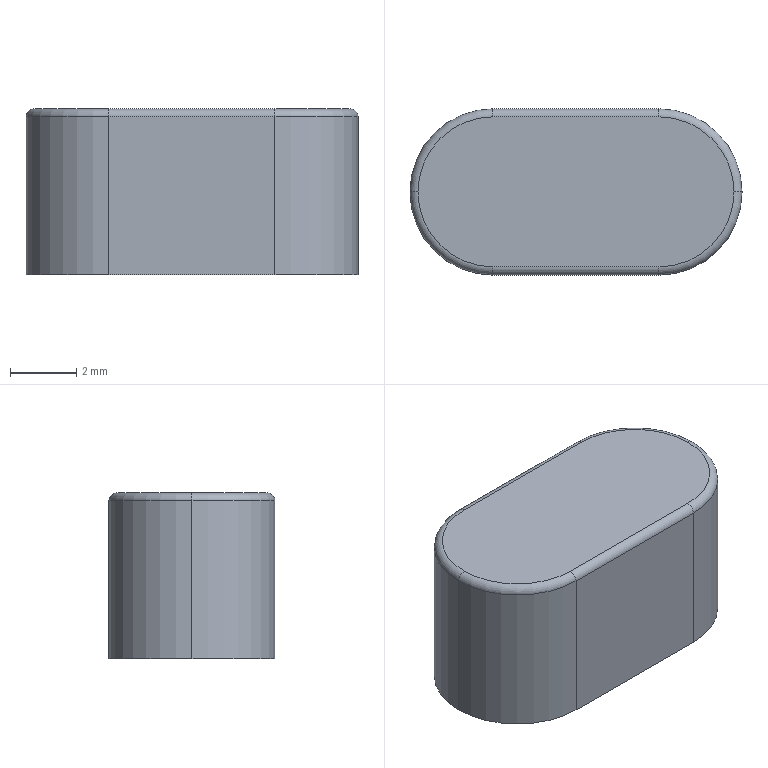Part | NX | features BLEND 2, DATUM_CSYS 2, EXTRUDE 1, SKETCH 1 | 1 solid | 14 faces | box 10 x 5 x 5 mm | volume 222.861 mm3 | cylinder 6 | plane 4 | torus 4 | commonest cylinder face diameters 5 x4 0.48 x2
STEP:
#1=CARTESIAN_POINT('',(2.5,-2.5,0.));
#2=VERTEX_POINT('',#1);
#3=CARTESIAN_POINT('',(2.5,-2.5,4.76));
#4=VERTEX_POINT('',#3);
#5=CARTESIAN_POINT('',(2.5,-2.5,5.));
#6=DIRECTION('',(0.,0.,-1.));
#7=VECTOR('',#6,1000.);
#8=LINE('',#5,#7);
#9=EDGE_CURVE('',#2,#4,#8,.F.);
#10=ORIENTED_EDGE('',*,*,#9,.T.);
#11=CARTESIAN_POINT('',(-2.5,-2.5,4.76));
#12=VERTEX_POINT('',#11);
#13=CARTESIAN_POINT('',(-2.5,-2.5,4.76));
#14=DIRECTION('',(1.,0.,0.));
#15=VECTOR('',#14,1000.);
#16=LINE('',#13,#15);
#17=EDGE_CURVE('',#4,#12,#16,.F.);
#18=ORIENTED_EDGE('',*,*,#17,.T.);
#19=CARTESIAN_POINT('',(-2.5,-2.5,0.));
#20=VERTEX_POINT('',#19);
#21=CARTESIAN_POINT('',(-2.5,-2.5,5.));
#22=DIRECTION('',(0.,0.,-1.));
#23=VECTOR('',#22,1000.);
#24=LINE('',#21,#23);
#25=EDGE_CURVE('',#12,#20,#24,.T.);
#26=ORIENTED_EDGE('',*,*,#25,.T.);
#27=CARTESIAN_POINT('',(-5.,-2.5,0.));
#28=DIRECTION('',(1.,0.,0.));
#29=VECTOR('',#28,1000.);
#30=LINE('',#27,#29);
#31=EDGE_CURVE('',#20,#2,#30,.T.);
#32=ORIENTED_EDGE('',*,*,#31,.T.);
#33=EDGE_LOOP('',(#10,#18,#26,#32));
#34=FACE_BOUND('',#33,.T.);
#35=CARTESIAN_POINT('',(-5.,-2.5,5.));
#36=DIRECTION('',(0.,1.,0.));
#37=DIRECTION('',(0.,0.,1.));
#38=AXIS2_PLACEMENT_3D('',#35,#36,#37);
#39=PLANE('',#38);
#40=ADVANCED_FACE('',(#34),#39,.F.);
#41=CARTESIAN_POINT('',(-2.5,2.5,0.));
#42=VERTEX_POINT('',#41);
#43=CARTESIAN_POINT('',(-2.5,2.5,4.76));
#44=VERTEX_POINT('',#43);
#45=CARTESIAN_POINT('',(-2.5,2.5,5.));
#46=DIRECTION('',(0.,0.,-1.));
#47=VECTOR('',#46,1000.);
#48=LINE('',#45,#47);
#49=EDGE_CURVE('',#42,#44,#48,.F.);
#50=ORIENTED_EDGE('',*,*,#49,.T.);
#51=CARTESIAN_POINT('',(2.5,2.5,4.76));
#52=VERTEX_POINT('',#51);
#53=CARTESIAN_POINT('',(2.5,2.5,4.76));
#54=DIRECTION('',(-1.,0.,0.));
#55=VECTOR('',#54,1000.);
#56=LINE('',#53,#55);
#57=EDGE_CURVE('',#44,#52,#56,.F.);
#58=ORIENTED_EDGE('',*,*,#57,.T.);
#59=CARTESIAN_POINT('',(2.5,2.5,0.));
#60=VERTEX_POINT('',#59);
#61=CARTESIAN_POINT('',(2.5,2.5,5.));
#62=DIRECTION('',(0.,0.,-1.));
#63=VECTOR('',#62,1000.);
#64=LINE('',#61,#63);
#65=EDGE_CURVE('',#52,#60,#64,.T.);
#66=ORIENTED_EDGE('',*,*,#65,.T.);
#67=CARTESIAN_POINT('',(5.,2.5,0.));
#68=DIRECTION('',(-1.,0.,0.));
#69=VECTOR('',#68,1000.);
#70=LINE('',#67,#69);
#71=EDGE_CURVE('',#60,#42,#70,.T.);
#72=ORIENTED_EDGE('',*,*,#71,.T.);
#73=EDGE_LOOP('',(#50,#58,#66,#72));
#74=FACE_BOUND('',#73,.T.);
#75=CARTESIAN_POINT('',(5.,2.5,5.));
#76=DIRECTION('',(0.,-1.,0.));
#77=DIRECTION('',(0.,0.,-1.));
#78=AXIS2_PLACEMENT_3D('',#75,#76,#77);
#79=PLANE('',#78);
#80=ADVANCED_FACE('',(#74),#79,.F.);
#81=CARTESIAN_POINT('',(2.5,2.26,5.));
#82=VERTEX_POINT('',#81);
#83=CARTESIAN_POINT('',(-2.5,2.26,5.));
#84=VERTEX_POINT('',#83);
#85=CARTESIAN_POINT('',(-2.5,2.26,5.));
#86=DIRECTION('',(-1.,0.,0.));
#87=VECTOR('',#86,1000.);
#88=LINE('',#85,#87);
#89=EDGE_CURVE('',#82,#84,#88,.T.);
#90=ORIENTED_EDGE('',*,*,#89,.T.);
#91=CARTESIAN_POINT('',(-4.76,0.,5.));
#92=VERTEX_POINT('',#91);
#93=CARTESIAN_POINT('',(-2.5,0.,5.));
#94=DIRECTION('',(0.,0.,1.));
#95=DIRECTION('',(1.,0.,0.));
#96=AXIS2_PLACEMENT_3D('',#93,#94,#95);
#97=CIRCLE('',#96,2.26);
#98=EDGE_CURVE('',#84,#92,#97,.T.);
#99=ORIENTED_EDGE('',*,*,#98,.T.);
#100=CARTESIAN_POINT('',(-2.5,-2.26,5.));
#101=VERTEX_POINT('',#100);
#102=CARTESIAN_POINT('',(-2.5,0.,5.));
#103=DIRECTION('',(0.,0.,1.));
#104=DIRECTION('',(1.,0.,0.));
#105=AXIS2_PLACEMENT_3D('',#102,#103,#104);
#106=CIRCLE('',#105,2.26);
#107=EDGE_CURVE('',#92,#101,#106,.T.);
#108=ORIENTED_EDGE('',*,*,#107,.T.);
#109=CARTESIAN_POINT('',(2.5,-2.26,5.));
#110=VERTEX_POINT('',#109);
#111=CARTESIAN_POINT('',(2.5,-2.26,5.));
#112=DIRECTION('',(1.,0.,0.));
#113=VECTOR('',#112,1000.);
#114=LINE('',#111,#113);
#115=EDGE_CURVE('',#101,#110,#114,.T.);
#116=ORIENTED_EDGE('',*,*,#115,.T.);
#117=CARTESIAN_POINT('',(4.76,0.,5.));
#118=VERTEX_POINT('',#117);
#119=CARTESIAN_POINT('',(2.5,0.,5.));
#120=DIRECTION('',(0.,0.,1.));
#121=DIRECTION('',(1.,0.,0.));
#122=AXIS2_PLACEMENT_3D('',#119,#120,#121);
#123=CIRCLE('',#122,2.26);
#124=EDGE_CURVE('',#110,#118,#123,.T.);
#125=ORIENTED_EDGE('',*,*,#124,.T.);
#126=CARTESIAN_POINT('',(2.5,0.,5.));
#127=DIRECTION('',(0.,0.,1.));
#128=DIRECTION('',(1.,0.,0.));
#129=AXIS2_PLACEMENT_3D('',#126,#127,#128);
#130=CIRCLE('',#129,2.26);
#131=EDGE_CURVE('',#118,#82,#130,.T.);
#132=ORIENTED_EDGE('',*,*,#131,.T.);
#133=EDGE_LOOP('',(#90,#99,#108,#116,#125,#132));
#134=FACE_BOUND('',#133,.T.);
#135=CARTESIAN_POINT('',(0.,0.,5.));
#136=DIRECTION('',(0.,0.,1.));
#137=DIRECTION('',(1.,0.,0.));
#138=AXIS2_PLACEMENT_3D('',#135,#136,#137);
#139=PLANE('',#138);
#140=ADVANCED_FACE('',(#134),#139,.T.);
#141=CARTESIAN_POINT('',(-5.,0.,0.));
#142=VERTEX_POINT('',#141);
#143=CARTESIAN_POINT('',(-2.5,0.,0.));
#144=DIRECTION('',(0.,0.,1.));
#145=DIRECTION('',(1.,0.,0.));
#146=AXIS2_PLACEMENT_3D('',#143,#144,#145);
#147=CIRCLE('',#146,2.5);
#148=EDGE_CURVE('',#20,#142,#147,.F.);
#149=ORIENTED_EDGE('',*,*,#148,.T.);
#150=CARTESIAN_POINT('',(-2.5,0.,0.));
#151=DIRECTION('',(0.,0.,1.));
#152=DIRECTION('',(1.,0.,0.));
#153=AXIS2_PLACEMENT_3D('',#150,#151,#152);
#154=CIRCLE('',#153,2.5);
#155=EDGE_CURVE('',#142,#42,#154,.F.);
#156=ORIENTED_EDGE('',*,*,#155,.T.);
#157=ORIENTED_EDGE('',*,*,#71,.F.);
#158=CARTESIAN_POINT('',(5.,0.,0.));
#159=VERTEX_POINT('',#158);
#160=CARTESIAN_POINT('',(2.5,0.,0.));
#161=DIRECTION('',(0.,0.,1.));
#162=DIRECTION('',(1.,0.,0.));
#163=AXIS2_PLACEMENT_3D('',#160,#161,#162);
#164=CIRCLE('',#163,2.5);
#165=EDGE_CURVE('',#60,#159,#164,.F.);
#166=ORIENTED_EDGE('',*,*,#165,.T.);
#167=CARTESIAN_POINT('',(2.5,0.,0.));
#168=DIRECTION('',(0.,0.,1.));
#169=DIRECTION('',(1.,0.,0.));
#170=AXIS2_PLACEMENT_3D('',#167,#168,#169);
#171=CIRCLE('',#170,2.5);
#172=EDGE_CURVE('',#159,#2,#171,.F.);
#173=ORIENTED_EDGE('',*,*,#172,.T.);
#174=ORIENTED_EDGE('',*,*,#31,.F.);
#175=EDGE_LOOP('',(#149,#156,#157,#166,#173,#174));
#176=FACE_BOUND('',#175,.T.);
#177=CARTESIAN_POINT('',(0.,0.,0.));
#178=DIRECTION('',(0.,0.,1.));
#179=DIRECTION('',(1.,0.,0.));
#180=AXIS2_PLACEMENT_3D('',#177,#178,#179);
#181=PLANE('',#180);
#182=ADVANCED_FACE('',(#176),#181,.F.);
#183=ORIENTED_EDGE('',*,*,#25,.F.);
#184=CARTESIAN_POINT('',(-5.,0.,4.76));
#185=VERTEX_POINT('',#184);
#186=CARTESIAN_POINT('',(-2.5,0.,4.76));
#187=DIRECTION('',(0.,0.,1.));
#188=DIRECTION('',(1.,0.,0.));
#189=AXIS2_PLACEMENT_3D('',#186,#187,#188);
#190=CIRCLE('',#189,2.5);
#191=EDGE_CURVE('',#12,#185,#190,.F.);
#192=ORIENTED_EDGE('',*,*,#191,.T.);
#193=CARTESIAN_POINT('',(-5.,0.,5.));
#194=DIRECTION('',(0.,0.,-1.));
#195=VECTOR('',#194,1000.);
#196=LINE('',#193,#195);
#197=EDGE_CURVE('',#142,#185,#196,.F.);
#198=ORIENTED_EDGE('',*,*,#197,.F.);
#199=ORIENTED_EDGE('',*,*,#148,.F.);
#200=EDGE_LOOP('',(#183,#192,#198,#199));
#201=FACE_BOUND('',#200,.T.);
#202=CARTESIAN_POINT('',(-2.5,0.,5.));
#203=DIRECTION('',(0.,0.,-1.));
#204=DIRECTION('',(-1.,0.,0.));
#205=AXIS2_PLACEMENT_3D('',#202,#203,#204);
#206=CYLINDRICAL_SURFACE('',#205,2.5);
#207=ADVANCED_FACE('',(#201),#206,.T.);
#208=ORIENTED_EDGE('',*,*,#197,.T.);
#209=CARTESIAN_POINT('',(-2.5,0.,4.76));
#210=DIRECTION('',(0.,0.,1.));
#211=DIRECTION('',(1.,0.,0.));
#212=AXIS2_PLACEMENT_3D('',#209,#210,#211);
#213=CIRCLE('',#212,2.5);
#214=EDGE_CURVE('',#185,#44,#213,.F.);
#215=ORIENTED_EDGE('',*,*,#214,.T.);
#216=ORIENTED_EDGE('',*,*,#49,.F.);
#217=ORIENTED_EDGE('',*,*,#155,.F.);
#218=EDGE_LOOP('',(#208,#215,#216,#217));
#219=FACE_BOUND('',#218,.T.);
#220=CARTESIAN_POINT('',(-2.5,0.,5.));
#221=DIRECTION('',(0.,0.,-1.));
#222=DIRECTION('',(-1.,0.,0.));
#223=AXIS2_PLACEMENT_3D('',#220,#221,#222);
#224=CYLINDRICAL_SURFACE('',#223,2.5);
#225=ADVANCED_FACE('',(#219),#224,.T.);
#226=CARTESIAN_POINT('',(5.,0.,4.76));
#227=VERTEX_POINT('',#226);
#228=CARTESIAN_POINT('',(5.,0.,5.));
#229=DIRECTION('',(0.,0.,-1.));
#230=VECTOR('',#229,1000.);
#231=LINE('',#228,#230);
#232=EDGE_CURVE('',#227,#159,#231,.T.);
#233=ORIENTED_EDGE('',*,*,#232,.F.);
#234=CARTESIAN_POINT('',(2.5,0.,4.76));
#235=DIRECTION('',(0.,0.,1.));
#236=DIRECTION('',(1.,0.,0.));
#237=AXIS2_PLACEMENT_3D('',#234,#235,#236);
#238=CIRCLE('',#237,2.5);
#239=EDGE_CURVE('',#227,#4,#238,.F.);
#240=ORIENTED_EDGE('',*,*,#239,.T.);
#241=ORIENTED_EDGE('',*,*,#9,.F.);
#242=ORIENTED_EDGE('',*,*,#172,.F.);
#243=EDGE_LOOP('',(#233,#240,#241,#242));
#244=FACE_BOUND('',#243,.T.);
#245=CARTESIAN_POINT('',(2.5,0.,5.));
#246=DIRECTION('',(0.,0.,-1.));
#247=DIRECTION('',(-1.,0.,0.));
#248=AXIS2_PLACEMENT_3D('',#245,#246,#247);
#249=CYLINDRICAL_SURFACE('',#248,2.5);
#250=ADVANCED_FACE('',(#244),#249,.T.);
#251=ORIENTED_EDGE('',*,*,#65,.F.);
#252=CARTESIAN_POINT('',(2.5,0.,4.76));
#253=DIRECTION('',(0.,0.,1.));
#254=DIRECTION('',(1.,0.,0.));
#255=AXIS2_PLACEMENT_3D('',#252,#253,#254);
#256=CIRCLE('',#255,2.5);
#257=EDGE_CURVE('',#52,#227,#256,.F.);
#258=ORIENTED_EDGE('',*,*,#257,.T.);
#259=ORIENTED_EDGE('',*,*,#232,.T.);
#260=ORIENTED_EDGE('',*,*,#165,.F.);
#261=EDGE_LOOP('',(#251,#258,#259,#260));
#262=FACE_BOUND('',#261,.T.);
#263=CARTESIAN_POINT('',(2.5,0.,5.));
#264=DIRECTION('',(0.,0.,-1.));
#265=DIRECTION('',(-1.,0.,0.));
#266=AXIS2_PLACEMENT_3D('',#263,#264,#265);
#267=CYLINDRICAL_SURFACE('',#266,2.5);
#268=ADVANCED_FACE('',(#262),#267,.T.);
#269=CARTESIAN_POINT('',(2.5,-2.26,4.76));
#270=DIRECTION('',(-1.,0.,0.));
#271=DIRECTION('',(0.,0.,1.));
#272=AXIS2_PLACEMENT_3D('',#269,#270,#271);
#273=CIRCLE('',#272,0.24);
#274=EDGE_CURVE('',#4,#110,#273,.T.);
#275=ORIENTED_EDGE('',*,*,#274,.F.);
#276=ORIENTED_EDGE('',*,*,#239,.F.);
#277=CARTESIAN_POINT('',(4.76,0.,4.76));
#278=DIRECTION('',(0.,1.,0.));
#279=DIRECTION('',(-1.,0.,0.));
#280=AXIS2_PLACEMENT_3D('',#277,#278,#279);
#281=CIRCLE('',#280,0.24);
#282=EDGE_CURVE('',#118,#227,#281,.T.);
#283=ORIENTED_EDGE('',*,*,#282,.F.);
#284=ORIENTED_EDGE('',*,*,#124,.F.);
#285=EDGE_LOOP('',(#275,#276,#283,#284));
#286=FACE_BOUND('',#285,.T.);
#287=CARTESIAN_POINT('',(2.5,0.,4.76));
#288=DIRECTION('',(0.,0.,1.));
#289=DIRECTION('',(1.,0.,0.));
#290=AXIS2_PLACEMENT_3D('',#287,#288,#289);
#291=TOROIDAL_SURFACE('',#290,2.26,0.24);
#292=ADVANCED_FACE('',(#286),#291,.T.);
#293=ORIENTED_EDGE('',*,*,#282,.T.);
#294=ORIENTED_EDGE('',*,*,#257,.F.);
#295=CARTESIAN_POINT('',(2.5,2.26,4.76));
#296=DIRECTION('',(-1.,0.,0.));
#297=DIRECTION('',(0.,0.,1.));
#298=AXIS2_PLACEMENT_3D('',#295,#296,#297);
#299=CIRCLE('',#298,0.24);
#300=EDGE_CURVE('',#82,#52,#299,.T.);
#301=ORIENTED_EDGE('',*,*,#300,.F.);
#302=ORIENTED_EDGE('',*,*,#131,.F.);
#303=EDGE_LOOP('',(#293,#294,#301,#302));
#304=FACE_BOUND('',#303,.T.);
#305=CARTESIAN_POINT('',(2.5,0.,4.76));
#306=DIRECTION('',(0.,0.,1.));
#307=DIRECTION('',(1.,0.,0.));
#308=AXIS2_PLACEMENT_3D('',#305,#306,#307);
#309=TOROIDAL_SURFACE('',#308,2.26,0.24);
#310=ADVANCED_FACE('',(#304),#309,.T.);
#311=ORIENTED_EDGE('',*,*,#274,.T.);
#312=ORIENTED_EDGE('',*,*,#115,.F.);
#313=CARTESIAN_POINT('',(-2.5,-2.26,4.76));
#314=DIRECTION('',(-1.,0.,0.));
#315=DIRECTION('',(0.,0.,1.));
#316=AXIS2_PLACEMENT_3D('',#313,#314,#315);
#317=CIRCLE('',#316,0.24);
#318=EDGE_CURVE('',#12,#101,#317,.T.);
#319=ORIENTED_EDGE('',*,*,#318,.F.);
#320=ORIENTED_EDGE('',*,*,#17,.F.);
#321=EDGE_LOOP('',(#311,#312,#319,#320));
#322=FACE_BOUND('',#321,.T.);
#323=CARTESIAN_POINT('',(0.,-2.26,4.76));
#324=DIRECTION('',(-1.,0.,0.));
#325=DIRECTION('',(0.,0.,1.));
#326=AXIS2_PLACEMENT_3D('',#323,#324,#325);
#327=CYLINDRICAL_SURFACE('',#326,0.24);
#328=ADVANCED_FACE('',(#322),#327,.T.);
#329=ORIENTED_EDGE('',*,*,#300,.T.);
#330=ORIENTED_EDGE('',*,*,#57,.F.);
#331=CARTESIAN_POINT('',(-2.5,2.26,4.76));
#332=DIRECTION('',(-1.,0.,0.));
#333=DIRECTION('',(0.,0.,1.));
#334=AXIS2_PLACEMENT_3D('',#331,#332,#333);
#335=CIRCLE('',#334,0.24);
#336=EDGE_CURVE('',#84,#44,#335,.T.);
#337=ORIENTED_EDGE('',*,*,#336,.F.);
#338=ORIENTED_EDGE('',*,*,#89,.F.);
#339=EDGE_LOOP('',(#329,#330,#337,#338));
#340=FACE_BOUND('',#339,.T.);
#341=CARTESIAN_POINT('',(0.,2.26,4.76));
#342=DIRECTION('',(1.,0.,0.));
#343=DIRECTION('',(0.,0.,-1.));
#344=AXIS2_PLACEMENT_3D('',#341,#342,#343);
#345=CYLINDRICAL_SURFACE('',#344,0.24);
#346=ADVANCED_FACE('',(#340),#345,.T.);
#347=ORIENTED_EDGE('',*,*,#318,.T.);
#348=ORIENTED_EDGE('',*,*,#107,.F.);
#349=CARTESIAN_POINT('',(-4.76,0.,4.76));
#350=DIRECTION('',(0.,1.,0.));
#351=DIRECTION('',(0.,0.,1.));
#352=AXIS2_PLACEMENT_3D('',#349,#350,#351);
#353=CIRCLE('',#352,0.24);
#354=EDGE_CURVE('',#185,#92,#353,.T.);
#355=ORIENTED_EDGE('',*,*,#354,.F.);
#356=ORIENTED_EDGE('',*,*,#191,.F.);
#357=EDGE_LOOP('',(#347,#348,#355,#356));
#358=FACE_BOUND('',#357,.T.);
#359=CARTESIAN_POINT('',(-2.5,0.,4.76));
#360=DIRECTION('',(0.,0.,1.));
#361=DIRECTION('',(1.,0.,0.));
#362=AXIS2_PLACEMENT_3D('',#359,#360,#361);
#363=TOROIDAL_SURFACE('',#362,2.26,0.24);
#364=ADVANCED_FACE('',(#358),#363,.T.);
#365=ORIENTED_EDGE('',*,*,#336,.T.);
#366=ORIENTED_EDGE('',*,*,#214,.F.);
#367=ORIENTED_EDGE('',*,*,#354,.T.);
#368=ORIENTED_EDGE('',*,*,#98,.F.);
#369=EDGE_LOOP('',(#365,#366,#367,#368));
#370=FACE_BOUND('',#369,.T.);
#371=CARTESIAN_POINT('',(-2.5,0.,4.76));
#372=DIRECTION('',(0.,0.,1.));
#373=DIRECTION('',(1.,0.,0.));
#374=AXIS2_PLACEMENT_3D('',#371,#372,#373);
#375=TOROIDAL_SURFACE('',#374,2.26,0.24);
#376=ADVANCED_FACE('',(#370),#375,.T.);
#377=CLOSED_SHELL('',(#40,#80,#140,#182,#207,#225,#250,#268,#292,#310,#328,#346,#364,#376));
#378=MANIFOLD_SOLID_BREP('',#377);
#379=(LENGTH_UNIT()NAMED_UNIT(*)SI_UNIT(.MILLI.,.METRE.));
#380=UNCERTAINTY_MEASURE_WITH_UNIT(LENGTH_MEASURE(0.00001),#379,'','');
#381=(NAMED_UNIT(*)PLANE_ANGLE_UNIT()SI_UNIT($,.RADIAN.));
#382=(NAMED_UNIT(*)SI_UNIT($,.STERADIAN.)SOLID_ANGLE_UNIT());
#383=(GEOMETRIC_REPRESENTATION_CONTEXT(3)GLOBAL_UNCERTAINTY_ASSIGNED_CONTEXT((#380))GLOBAL_UNIT_ASSIGNED_CONTEXT((#379,#381,#382))REPRESENTATION_CONTEXT('',''));
#384=ADVANCED_BREP_SHAPE_REPRESENTATION('',(#378),#383);